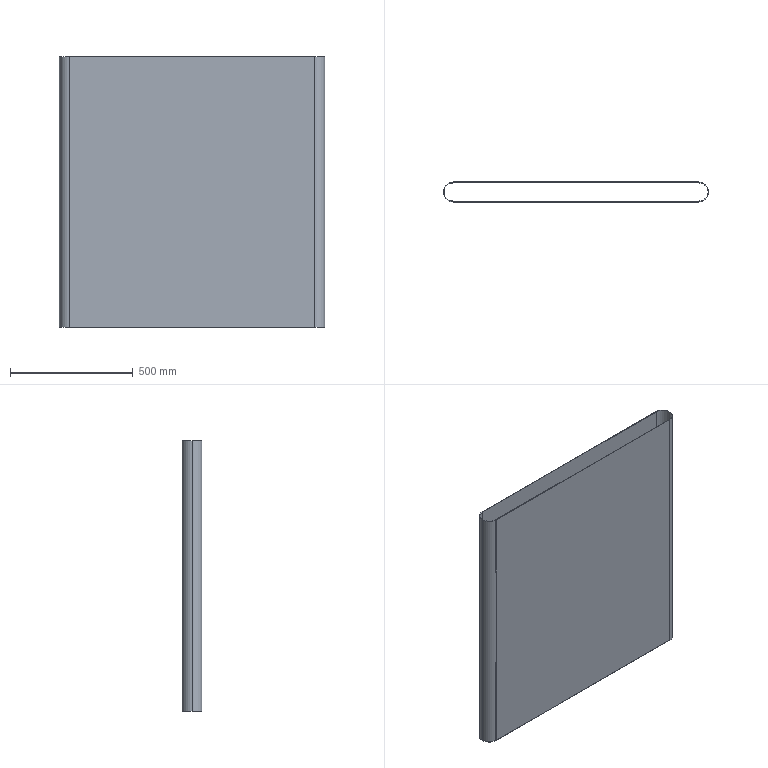Part | SolidWorks | features ExtruThin 1 | 1 solid | 12 faces | box 1080 x 80 x 1100 mm | volume 4939097 mm3 | cylinder 6 | plane 6 | commonest cylinder face diameters 76 x3 80 x3
STEP:
#1=CARTESIAN_POINT('',(-500.,38.,550.));
#2=VERTEX_POINT('',#1);
#3=CARTESIAN_POINT('',(-538.,0.,550.));
#4=VERTEX_POINT('',#3);
#5=CARTESIAN_POINT('',(-500.,0.,550.));
#6=DIRECTION('',(0.,0.,1.));
#7=DIRECTION('',(1.,0.,0.));
#8=AXIS2_PLACEMENT_3D('',#5,#6,#7);
#9=CIRCLE('',#8,38.);
#10=EDGE_CURVE('',#2,#4,#9,.T.);
#11=ORIENTED_EDGE('',*,*,#10,.T.);
#12=CARTESIAN_POINT('',(-538.,0.,-550.));
#13=VERTEX_POINT('',#12);
#14=CARTESIAN_POINT('',(-538.,0.,550.));
#15=DIRECTION('',(0.,0.,-1.));
#16=VECTOR('',#15,1000.);
#17=LINE('',#14,#16);
#18=EDGE_CURVE('',#4,#13,#17,.T.);
#19=ORIENTED_EDGE('',*,*,#18,.T.);
#20=CARTESIAN_POINT('',(-500.,38.,-550.));
#21=VERTEX_POINT('',#20);
#22=CARTESIAN_POINT('',(-500.,0.,-550.));
#23=DIRECTION('',(0.,0.,1.));
#24=DIRECTION('',(1.,0.,0.));
#25=AXIS2_PLACEMENT_3D('',#22,#23,#24);
#26=CIRCLE('',#25,38.);
#27=EDGE_CURVE('',#21,#13,#26,.T.);
#28=ORIENTED_EDGE('',*,*,#27,.F.);
#29=CARTESIAN_POINT('',(-500.,38.,550.));
#30=DIRECTION('',(0.,0.,-1.));
#31=VECTOR('',#30,1000.);
#32=LINE('',#29,#31);
#33=EDGE_CURVE('',#2,#21,#32,.T.);
#34=ORIENTED_EDGE('',*,*,#33,.F.);
#35=EDGE_LOOP('',(#11,#19,#28,#34));
#36=FACE_OUTER_BOUND('',#35,.T.);
#37=CARTESIAN_POINT('',(-500.,0.,550.));
#38=DIRECTION('',(0.,0.,-1.));
#39=DIRECTION('',(-1.,0.,0.));
#40=AXIS2_PLACEMENT_3D('',#37,#38,#39);
#41=CYLINDRICAL_SURFACE('',#40,38.);
#42=ADVANCED_FACE('',(#36),#41,.F.);
#43=CARTESIAN_POINT('',(-540.,0.,550.));
#44=VERTEX_POINT('',#43);
#45=CARTESIAN_POINT('',(-500.,-40.,550.));
#46=VERTEX_POINT('',#45);
#47=CARTESIAN_POINT('',(-500.,0.,550.));
#48=DIRECTION('',(0.,0.,1.));
#49=DIRECTION('',(1.,0.,0.));
#50=AXIS2_PLACEMENT_3D('',#47,#48,#49);
#51=CIRCLE('',#50,40.);
#52=EDGE_CURVE('',#44,#46,#51,.T.);
#53=ORIENTED_EDGE('',*,*,#52,.F.);
#54=CARTESIAN_POINT('',(-540.,0.,-550.));
#55=VERTEX_POINT('',#54);
#56=CARTESIAN_POINT('',(-540.,0.,550.));
#57=DIRECTION('',(0.,0.,-1.));
#58=VECTOR('',#57,1000.);
#59=LINE('',#56,#58);
#60=EDGE_CURVE('',#44,#55,#59,.T.);
#61=ORIENTED_EDGE('',*,*,#60,.T.);
#62=CARTESIAN_POINT('',(-500.,-40.,-550.));
#63=VERTEX_POINT('',#62);
#64=CARTESIAN_POINT('',(-500.,0.,-550.));
#65=DIRECTION('',(0.,0.,1.));
#66=DIRECTION('',(1.,0.,0.));
#67=AXIS2_PLACEMENT_3D('',#64,#65,#66);
#68=CIRCLE('',#67,40.);
#69=EDGE_CURVE('',#55,#63,#68,.T.);
#70=ORIENTED_EDGE('',*,*,#69,.T.);
#71=CARTESIAN_POINT('',(-500.,-40.,550.));
#72=DIRECTION('',(0.,0.,-1.));
#73=VECTOR('',#72,1000.);
#74=LINE('',#71,#73);
#75=EDGE_CURVE('',#46,#63,#74,.T.);
#76=ORIENTED_EDGE('',*,*,#75,.F.);
#77=EDGE_LOOP('',(#53,#61,#70,#76));
#78=FACE_OUTER_BOUND('',#77,.T.);
#79=CARTESIAN_POINT('',(-500.,0.,550.));
#80=DIRECTION('',(0.,0.,-1.));
#81=DIRECTION('',(-1.,0.,0.));
#82=AXIS2_PLACEMENT_3D('',#79,#80,#81);
#83=CYLINDRICAL_SURFACE('',#82,40.);
#84=ADVANCED_FACE('',(#78),#83,.T.);
#85=CARTESIAN_POINT('',(-500.,40.,550.));
#86=VERTEX_POINT('',#85);
#87=CARTESIAN_POINT('',(-500.,0.,550.));
#88=DIRECTION('',(0.,0.,1.));
#89=DIRECTION('',(1.,0.,0.));
#90=AXIS2_PLACEMENT_3D('',#87,#88,#89);
#91=CIRCLE('',#90,40.);
#92=EDGE_CURVE('',#86,#44,#91,.T.);
#93=ORIENTED_EDGE('',*,*,#92,.T.);
#94=ORIENTED_EDGE('',*,*,#52,.T.);
#95=CARTESIAN_POINT('',(500.,-40.,550.));
#96=VERTEX_POINT('',#95);
#97=CARTESIAN_POINT('',(-500.,-40.,550.));
#98=DIRECTION('',(1.,0.,0.));
#99=VECTOR('',#98,1000.);
#100=LINE('',#97,#99);
#101=EDGE_CURVE('',#46,#96,#100,.T.);
#102=ORIENTED_EDGE('',*,*,#101,.T.);
#103=CARTESIAN_POINT('',(500.,40.,550.));
#104=VERTEX_POINT('',#103);
#105=CARTESIAN_POINT('',(500.,0.,550.));
#106=DIRECTION('',(0.,0.,1.));
#107=DIRECTION('',(1.,0.,0.));
#108=AXIS2_PLACEMENT_3D('',#105,#106,#107);
#109=CIRCLE('',#108,40.);
#110=EDGE_CURVE('',#96,#104,#109,.T.);
#111=ORIENTED_EDGE('',*,*,#110,.T.);
#112=CARTESIAN_POINT('',(-500.,40.,550.));
#113=DIRECTION('',(-1.,0.,0.));
#114=VECTOR('',#113,1000.);
#115=LINE('',#112,#114);
#116=EDGE_CURVE('',#104,#86,#115,.T.);
#117=ORIENTED_EDGE('',*,*,#116,.T.);
#118=EDGE_LOOP('',(#93,#94,#102,#111,#117));
#119=FACE_OUTER_BOUND('',#118,.T.);
#120=CARTESIAN_POINT('',(-500.,-38.,550.));
#121=VERTEX_POINT('',#120);
#122=CARTESIAN_POINT('',(500.,-38.,550.));
#123=VERTEX_POINT('',#122);
#124=CARTESIAN_POINT('',(-500.,-38.,550.));
#125=DIRECTION('',(1.,0.,0.));
#126=VECTOR('',#125,1000.);
#127=LINE('',#124,#126);
#128=EDGE_CURVE('',#121,#123,#127,.T.);
#129=ORIENTED_EDGE('',*,*,#128,.F.);
#130=CARTESIAN_POINT('',(-500.,0.,550.));
#131=DIRECTION('',(0.,0.,1.));
#132=DIRECTION('',(1.,0.,0.));
#133=AXIS2_PLACEMENT_3D('',#130,#131,#132);
#134=CIRCLE('',#133,38.);
#135=EDGE_CURVE('',#4,#121,#134,.T.);
#136=ORIENTED_EDGE('',*,*,#135,.F.);
#137=ORIENTED_EDGE('',*,*,#10,.F.);
#138=CARTESIAN_POINT('',(500.,38.,550.));
#139=VERTEX_POINT('',#138);
#140=CARTESIAN_POINT('',(-500.,38.,550.));
#141=DIRECTION('',(-1.,0.,0.));
#142=VECTOR('',#141,1000.);
#143=LINE('',#140,#142);
#144=EDGE_CURVE('',#139,#2,#143,.T.);
#145=ORIENTED_EDGE('',*,*,#144,.F.);
#146=CARTESIAN_POINT('',(500.,0.,550.));
#147=DIRECTION('',(0.,0.,1.));
#148=DIRECTION('',(1.,0.,0.));
#149=AXIS2_PLACEMENT_3D('',#146,#147,#148);
#150=CIRCLE('',#149,38.);
#151=EDGE_CURVE('',#123,#139,#150,.T.);
#152=ORIENTED_EDGE('',*,*,#151,.F.);
#153=EDGE_LOOP('',(#129,#136,#137,#145,#152));
#154=FACE_BOUND('',#153,.T.);
#155=CARTESIAN_POINT('',(-500.,0.,550.));
#156=DIRECTION('',(0.,0.,1.));
#157=DIRECTION('',(1.,0.,0.));
#158=AXIS2_PLACEMENT_3D('',#155,#156,#157);
#159=PLANE('',#158);
#160=ADVANCED_FACE('',(#119,#154),#159,.T.);
#161=CARTESIAN_POINT('',(-500.,40.,-550.));
#162=VERTEX_POINT('',#161);
#163=CARTESIAN_POINT('',(-500.,0.,-550.));
#164=DIRECTION('',(0.,0.,1.));
#165=DIRECTION('',(1.,0.,0.));
#166=AXIS2_PLACEMENT_3D('',#163,#164,#165);
#167=CIRCLE('',#166,40.);
#168=EDGE_CURVE('',#162,#55,#167,.T.);
#169=ORIENTED_EDGE('',*,*,#168,.F.);
#170=CARTESIAN_POINT('',(500.,40.,-550.));
#171=VERTEX_POINT('',#170);
#172=CARTESIAN_POINT('',(-500.,40.,-550.));
#173=DIRECTION('',(-1.,0.,0.));
#174=VECTOR('',#173,1000.);
#175=LINE('',#172,#174);
#176=EDGE_CURVE('',#171,#162,#175,.T.);
#177=ORIENTED_EDGE('',*,*,#176,.F.);
#178=CARTESIAN_POINT('',(500.,-40.,-550.));
#179=VERTEX_POINT('',#178);
#180=CARTESIAN_POINT('',(500.,0.,-550.));
#181=DIRECTION('',(0.,0.,1.));
#182=DIRECTION('',(1.,0.,0.));
#183=AXIS2_PLACEMENT_3D('',#180,#181,#182);
#184=CIRCLE('',#183,40.);
#185=EDGE_CURVE('',#179,#171,#184,.T.);
#186=ORIENTED_EDGE('',*,*,#185,.F.);
#187=CARTESIAN_POINT('',(-500.,-40.,-550.));
#188=DIRECTION('',(1.,0.,0.));
#189=VECTOR('',#188,1000.);
#190=LINE('',#187,#189);
#191=EDGE_CURVE('',#63,#179,#190,.T.);
#192=ORIENTED_EDGE('',*,*,#191,.F.);
#193=ORIENTED_EDGE('',*,*,#69,.F.);
#194=EDGE_LOOP('',(#169,#177,#186,#192,#193));
#195=FACE_OUTER_BOUND('',#194,.T.);
#196=ORIENTED_EDGE('',*,*,#27,.T.);
#197=CARTESIAN_POINT('',(-500.,-38.,-550.));
#198=VERTEX_POINT('',#197);
#199=CARTESIAN_POINT('',(-500.,0.,-550.));
#200=DIRECTION('',(0.,0.,1.));
#201=DIRECTION('',(1.,0.,0.));
#202=AXIS2_PLACEMENT_3D('',#199,#200,#201);
#203=CIRCLE('',#202,38.);
#204=EDGE_CURVE('',#13,#198,#203,.T.);
#205=ORIENTED_EDGE('',*,*,#204,.T.);
#206=CARTESIAN_POINT('',(500.,-38.,-550.));
#207=VERTEX_POINT('',#206);
#208=CARTESIAN_POINT('',(-500.,-38.,-550.));
#209=DIRECTION('',(1.,0.,0.));
#210=VECTOR('',#209,1000.);
#211=LINE('',#208,#210);
#212=EDGE_CURVE('',#198,#207,#211,.T.);
#213=ORIENTED_EDGE('',*,*,#212,.T.);
#214=CARTESIAN_POINT('',(500.,38.,-550.));
#215=VERTEX_POINT('',#214);
#216=CARTESIAN_POINT('',(500.,0.,-550.));
#217=DIRECTION('',(0.,0.,1.));
#218=DIRECTION('',(1.,0.,0.));
#219=AXIS2_PLACEMENT_3D('',#216,#217,#218);
#220=CIRCLE('',#219,38.);
#221=EDGE_CURVE('',#207,#215,#220,.T.);
#222=ORIENTED_EDGE('',*,*,#221,.T.);
#223=CARTESIAN_POINT('',(-500.,38.,-550.));
#224=DIRECTION('',(-1.,0.,0.));
#225=VECTOR('',#224,1000.);
#226=LINE('',#223,#225);
#227=EDGE_CURVE('',#215,#21,#226,.T.);
#228=ORIENTED_EDGE('',*,*,#227,.T.);
#229=EDGE_LOOP('',(#196,#205,#213,#222,#228));
#230=FACE_BOUND('',#229,.T.);
#231=CARTESIAN_POINT('',(-500.,0.,-550.));
#232=DIRECTION('',(0.,0.,1.));
#233=DIRECTION('',(1.,0.,0.));
#234=AXIS2_PLACEMENT_3D('',#231,#232,#233);
#235=PLANE('',#234);
#236=ADVANCED_FACE('',(#195,#230),#235,.F.);
#237=ORIENTED_EDGE('',*,*,#60,.F.);
#238=ORIENTED_EDGE('',*,*,#92,.F.);
#239=CARTESIAN_POINT('',(-500.,40.,550.));
#240=DIRECTION('',(0.,0.,-1.));
#241=VECTOR('',#240,1000.);
#242=LINE('',#239,#241);
#243=EDGE_CURVE('',#86,#162,#242,.T.);
#244=ORIENTED_EDGE('',*,*,#243,.T.);
#245=ORIENTED_EDGE('',*,*,#168,.T.);
#246=EDGE_LOOP('',(#237,#238,#244,#245));
#247=FACE_OUTER_BOUND('',#246,.T.);
#248=CARTESIAN_POINT('',(-500.,0.,550.));
#249=DIRECTION('',(0.,0.,-1.));
#250=DIRECTION('',(-1.,0.,0.));
#251=AXIS2_PLACEMENT_3D('',#248,#249,#250);
#252=CYLINDRICAL_SURFACE('',#251,40.);
#253=ADVANCED_FACE('',(#247),#252,.T.);
#254=ORIENTED_EDGE('',*,*,#191,.T.);
#255=CARTESIAN_POINT('',(500.,-40.,550.));
#256=DIRECTION('',(0.,0.,-1.));
#257=VECTOR('',#256,1000.);
#258=LINE('',#255,#257);
#259=EDGE_CURVE('',#96,#179,#258,.T.);
#260=ORIENTED_EDGE('',*,*,#259,.F.);
#261=ORIENTED_EDGE('',*,*,#101,.F.);
#262=ORIENTED_EDGE('',*,*,#75,.T.);
#263=EDGE_LOOP('',(#254,#260,#261,#262));
#264=FACE_OUTER_BOUND('',#263,.T.);
#265=CARTESIAN_POINT('',(-500.,-40.,550.));
#266=DIRECTION('',(0.,1.,0.));
#267=DIRECTION('',(0.,0.,1.));
#268=AXIS2_PLACEMENT_3D('',#265,#266,#267);
#269=PLANE('',#268);
#270=ADVANCED_FACE('',(#264),#269,.F.);
#271=ORIENTED_EDGE('',*,*,#185,.T.);
#272=CARTESIAN_POINT('',(500.,40.,550.));
#273=DIRECTION('',(0.,0.,-1.));
#274=VECTOR('',#273,1000.);
#275=LINE('',#272,#274);
#276=EDGE_CURVE('',#104,#171,#275,.T.);
#277=ORIENTED_EDGE('',*,*,#276,.F.);
#278=ORIENTED_EDGE('',*,*,#110,.F.);
#279=ORIENTED_EDGE('',*,*,#259,.T.);
#280=EDGE_LOOP('',(#271,#277,#278,#279));
#281=FACE_OUTER_BOUND('',#280,.T.);
#282=CARTESIAN_POINT('',(500.,0.,550.));
#283=DIRECTION('',(0.,0.,-1.));
#284=DIRECTION('',(-1.,0.,0.));
#285=AXIS2_PLACEMENT_3D('',#282,#283,#284);
#286=CYLINDRICAL_SURFACE('',#285,40.);
#287=ADVANCED_FACE('',(#281),#286,.T.);
#288=ORIENTED_EDGE('',*,*,#176,.T.);
#289=ORIENTED_EDGE('',*,*,#243,.F.);
#290=ORIENTED_EDGE('',*,*,#116,.F.);
#291=ORIENTED_EDGE('',*,*,#276,.T.);
#292=EDGE_LOOP('',(#288,#289,#290,#291));
#293=FACE_OUTER_BOUND('',#292,.T.);
#294=CARTESIAN_POINT('',(-500.,40.,550.));
#295=DIRECTION('',(0.,-1.,0.));
#296=DIRECTION('',(0.,0.,-1.));
#297=AXIS2_PLACEMENT_3D('',#294,#295,#296);
#298=PLANE('',#297);
#299=ADVANCED_FACE('',(#293),#298,.F.);
#300=ORIENTED_EDGE('',*,*,#18,.F.);
#301=ORIENTED_EDGE('',*,*,#135,.T.);
#302=CARTESIAN_POINT('',(-500.,-38.,550.));
#303=DIRECTION('',(0.,0.,-1.));
#304=VECTOR('',#303,1000.);
#305=LINE('',#302,#304);
#306=EDGE_CURVE('',#121,#198,#305,.T.);
#307=ORIENTED_EDGE('',*,*,#306,.T.);
#308=ORIENTED_EDGE('',*,*,#204,.F.);
#309=EDGE_LOOP('',(#300,#301,#307,#308));
#310=FACE_OUTER_BOUND('',#309,.T.);
#311=CARTESIAN_POINT('',(-500.,0.,550.));
#312=DIRECTION('',(0.,0.,-1.));
#313=DIRECTION('',(-1.,0.,0.));
#314=AXIS2_PLACEMENT_3D('',#311,#312,#313);
#315=CYLINDRICAL_SURFACE('',#314,38.);
#316=ADVANCED_FACE('',(#310),#315,.F.);
#317=ORIENTED_EDGE('',*,*,#212,.F.);
#318=ORIENTED_EDGE('',*,*,#306,.F.);
#319=ORIENTED_EDGE('',*,*,#128,.T.);
#320=CARTESIAN_POINT('',(500.,-38.,550.));
#321=DIRECTION('',(0.,0.,-1.));
#322=VECTOR('',#321,1000.);
#323=LINE('',#320,#322);
#324=EDGE_CURVE('',#123,#207,#323,.T.);
#325=ORIENTED_EDGE('',*,*,#324,.T.);
#326=EDGE_LOOP('',(#317,#318,#319,#325));
#327=FACE_OUTER_BOUND('',#326,.T.);
#328=CARTESIAN_POINT('',(-500.,-38.,550.));
#329=DIRECTION('',(0.,1.,0.));
#330=DIRECTION('',(0.,0.,1.));
#331=AXIS2_PLACEMENT_3D('',#328,#329,#330);
#332=PLANE('',#331);
#333=ADVANCED_FACE('',(#327),#332,.T.);
#334=ORIENTED_EDGE('',*,*,#221,.F.);
#335=ORIENTED_EDGE('',*,*,#324,.F.);
#336=ORIENTED_EDGE('',*,*,#151,.T.);
#337=CARTESIAN_POINT('',(500.,38.,550.));
#338=DIRECTION('',(0.,0.,-1.));
#339=VECTOR('',#338,1000.);
#340=LINE('',#337,#339);
#341=EDGE_CURVE('',#139,#215,#340,.T.);
#342=ORIENTED_EDGE('',*,*,#341,.T.);
#343=EDGE_LOOP('',(#334,#335,#336,#342));
#344=FACE_OUTER_BOUND('',#343,.T.);
#345=CARTESIAN_POINT('',(500.,0.,550.));
#346=DIRECTION('',(0.,0.,-1.));
#347=DIRECTION('',(-1.,0.,0.));
#348=AXIS2_PLACEMENT_3D('',#345,#346,#347);
#349=CYLINDRICAL_SURFACE('',#348,38.);
#350=ADVANCED_FACE('',(#344),#349,.F.);
#351=ORIENTED_EDGE('',*,*,#227,.F.);
#352=ORIENTED_EDGE('',*,*,#341,.F.);
#353=ORIENTED_EDGE('',*,*,#144,.T.);
#354=ORIENTED_EDGE('',*,*,#33,.T.);
#355=EDGE_LOOP('',(#351,#352,#353,#354));
#356=FACE_OUTER_BOUND('',#355,.T.);
#357=CARTESIAN_POINT('',(-500.,38.,550.));
#358=DIRECTION('',(0.,-1.,0.));
#359=DIRECTION('',(0.,0.,-1.));
#360=AXIS2_PLACEMENT_3D('',#357,#358,#359);
#361=PLANE('',#360);
#362=ADVANCED_FACE('',(#356),#361,.T.);
#363=CLOSED_SHELL('',(#42,#84,#160,#236,#253,#270,#287,#299,#316,#333,#350,#362));
#364=MANIFOLD_SOLID_BREP('',#363);
#365=CARTESIAN_POINT('',(0.,0.,0.));
#366=DIRECTION('',(0.,0.,1.));
#367=DIRECTION('',(1.,0.,0.));
#368=AXIS2_PLACEMENT_3D('',#365,#366,#367);
#369=(LENGTH_UNIT()NAMED_UNIT(*)SI_UNIT(.MILLI.,.METRE.));
#370=UNCERTAINTY_MEASURE_WITH_UNIT(LENGTH_MEASURE(0.00001),#369,'','');
#371=(NAMED_UNIT(*)PLANE_ANGLE_UNIT()SI_UNIT($,.RADIAN.));
#372=(NAMED_UNIT(*)SI_UNIT($,.STERADIAN.)SOLID_ANGLE_UNIT());
#373=(GEOMETRIC_REPRESENTATION_CONTEXT(3)GLOBAL_UNCERTAINTY_ASSIGNED_CONTEXT((#370))GLOBAL_UNIT_ASSIGNED_CONTEXT((#369,#371,#372))REPRESENTATION_CONTEXT('',''));
#374=ADVANCED_BREP_SHAPE_REPRESENTATION('',(#364,#368),#373);